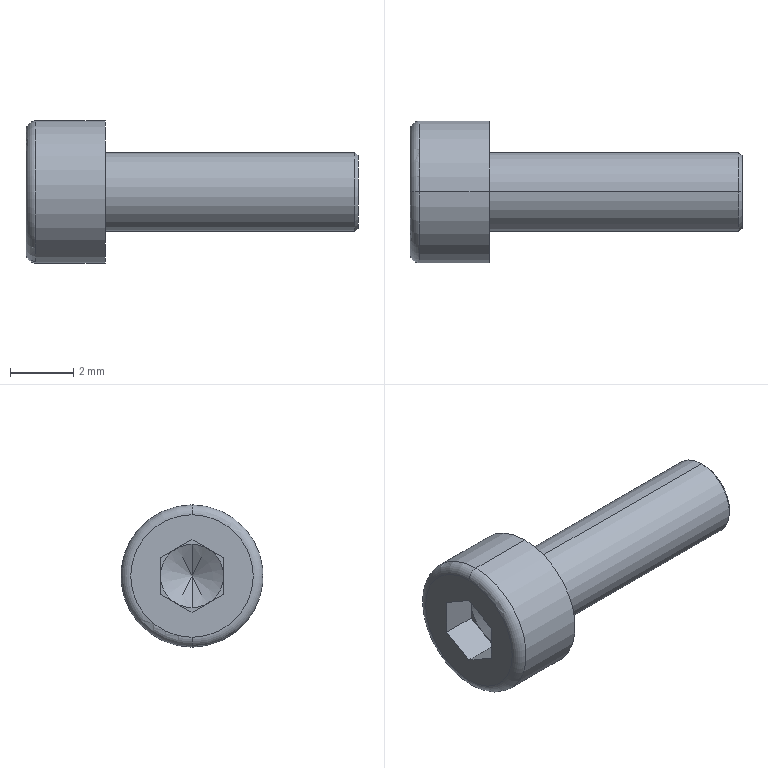Part | STEP file | hexagon socket head cap screws gb_GB_FASTENER_SCREWS_HSHCS M2.5X8-N | 1 solid | 25 faces | box 10.5 x 4.5 x 4.5 mm | volume 74.29 mm3 | plane 15 | cone 4 | cylinder 4 | torus 2 | commonest cylinder face diameters 2.5 x2 4.5 x2
STEP:
#1=CARTESIAN_POINT('',(10.5,0.,-1.15));
#2=VERTEX_POINT('',#1);
#3=CARTESIAN_POINT('',(10.5,0.,1.15));
#4=VERTEX_POINT('',#3);
#5=CARTESIAN_POINT('',(10.5,0.,0.));
#6=DIRECTION('',(1.,0.,0.));
#7=DIRECTION('',(0.,0.,-1.));
#8=AXIS2_PLACEMENT_3D('',#5,#6,#7);
#9=CIRCLE('',#8,1.15);
#10=EDGE_CURVE('',#2,#4,#9,.T.);
#11=ORIENTED_EDGE('',*,*,#10,.F.);
#12=CARTESIAN_POINT('',(10.4,0.,-1.25));
#13=VERTEX_POINT('',#12);
#14=CARTESIAN_POINT('',(10.5,0.,-1.15));
#15=DIRECTION('',(-0.7071,0.,-0.7071));
#16=VECTOR('',#15,1000.);
#17=LINE('',#14,#16);
#18=EDGE_CURVE('',#2,#13,#17,.T.);
#19=ORIENTED_EDGE('',*,*,#18,.T.);
#20=CARTESIAN_POINT('',(10.4,0.,1.25));
#21=VERTEX_POINT('',#20);
#22=CARTESIAN_POINT('',(10.4,0.,0.));
#23=DIRECTION('',(-1.,0.,0.));
#24=DIRECTION('',(0.,0.,-1.));
#25=AXIS2_PLACEMENT_3D('',#22,#23,#24);
#26=CIRCLE('',#25,1.25);
#27=EDGE_CURVE('',#21,#13,#26,.T.);
#28=ORIENTED_EDGE('',*,*,#27,.F.);
#29=CARTESIAN_POINT('',(10.5,0.,1.15));
#30=DIRECTION('',(-0.7071,0.,0.7071));
#31=VECTOR('',#30,1000.);
#32=LINE('',#29,#31);
#33=EDGE_CURVE('',#4,#21,#32,.T.);
#34=ORIENTED_EDGE('',*,*,#33,.F.);
#35=EDGE_LOOP('',(#11,#19,#28,#34));
#36=FACE_OUTER_BOUND('',#35,.T.);
#37=CARTESIAN_POINT('',(10.5,0.,0.));
#38=DIRECTION('',(-1.,0.,0.));
#39=DIRECTION('',(0.,0.,1.));
#40=AXIS2_PLACEMENT_3D('',#37,#38,#39);
#41=CONICAL_SURFACE('',#40,1.15,0.7854);
#42=ADVANCED_FACE('',(#36),#41,.T.);
#43=CARTESIAN_POINT('',(0.,0.,1.938));
#44=VERTEX_POINT('',#43);
#45=CARTESIAN_POINT('',(0.,0.,-1.938));
#46=VERTEX_POINT('',#45);
#47=CARTESIAN_POINT('',(0.,0.,0.));
#48=DIRECTION('',(-1.,0.,0.));
#49=DIRECTION('',(0.,0.,-1.));
#50=AXIS2_PLACEMENT_3D('',#47,#48,#49);
#51=CIRCLE('',#50,1.938);
#52=EDGE_CURVE('',#44,#46,#51,.T.);
#53=ORIENTED_EDGE('',*,*,#52,.F.);
#54=CARTESIAN_POINT('',(0.3125,0.,2.25));
#55=VERTEX_POINT('',#54);
#56=CARTESIAN_POINT('',(0.3125,0.,1.938));
#57=DIRECTION('',(0.,1.,0.));
#58=DIRECTION('',(0.,0.,1.));
#59=AXIS2_PLACEMENT_3D('',#56,#57,#58);
#60=CIRCLE('',#59,0.3125);
#61=EDGE_CURVE('',#44,#55,#60,.T.);
#62=ORIENTED_EDGE('',*,*,#61,.T.);
#63=CARTESIAN_POINT('',(0.3125,0.,-2.25));
#64=VERTEX_POINT('',#63);
#65=CARTESIAN_POINT('',(0.3125,0.,0.));
#66=DIRECTION('',(1.,0.,0.));
#67=DIRECTION('',(0.,0.,-1.));
#68=AXIS2_PLACEMENT_3D('',#65,#66,#67);
#69=CIRCLE('',#68,2.25);
#70=EDGE_CURVE('',#64,#55,#69,.T.);
#71=ORIENTED_EDGE('',*,*,#70,.F.);
#72=CARTESIAN_POINT('',(0.3125,0.,-1.938));
#73=DIRECTION('',(0.,-1.,0.));
#74=DIRECTION('',(0.,0.,-1.));
#75=AXIS2_PLACEMENT_3D('',#72,#73,#74);
#76=CIRCLE('',#75,0.3125);
#77=EDGE_CURVE('',#46,#64,#76,.T.);
#78=ORIENTED_EDGE('',*,*,#77,.F.);
#79=EDGE_LOOP('',(#53,#62,#71,#78));
#80=FACE_OUTER_BOUND('',#79,.T.);
#81=CARTESIAN_POINT('',(0.3125,0.,0.));
#82=DIRECTION('',(1.,0.,0.));
#83=DIRECTION('',(0.,0.,-1.));
#84=AXIS2_PLACEMENT_3D('',#81,#82,#83);
#85=TOROIDAL_SURFACE('',#84,1.938,0.3125);
#86=ADVANCED_FACE('',(#80),#85,.T.);
#87=CARTESIAN_POINT('',(1.677,0.,0.));
#88=VERTEX_POINT('',#87);
#89=CARTESIAN_POINT('',(1.1,0.,1.));
#90=VERTEX_POINT('',#89);
#91=CARTESIAN_POINT('',(1.1,0.,1.));
#92=DIRECTION('',(-0.5,0.,0.866));
#93=VECTOR('',#92,1000.);
#94=LINE('',#91,#93);
#95=EDGE_CURVE('',#88,#90,#94,.T.);
#96=ORIENTED_EDGE('',*,*,#95,.F.);
#97=CARTESIAN_POINT('',(1.1,0.,-1.));
#98=VERTEX_POINT('',#97);
#99=CARTESIAN_POINT('',(1.1,0.,-1.));
#100=DIRECTION('',(-0.5,0.,-0.866));
#101=VECTOR('',#100,1000.);
#102=LINE('',#99,#101);
#103=EDGE_CURVE('',#88,#98,#102,.T.);
#104=ORIENTED_EDGE('',*,*,#103,.T.);
#105=CARTESIAN_POINT('',(1.1,-0.5,-0.866));
#106=VERTEX_POINT('',#105);
#107=CARTESIAN_POINT('',(1.1,0.,0.));
#108=DIRECTION('',(-1.,0.,0.));
#109=DIRECTION('',(0.,0.,-1.));
#110=AXIS2_PLACEMENT_3D('',#107,#108,#109);
#111=CIRCLE('',#110,1.);
#112=EDGE_CURVE('',#98,#106,#111,.T.);
#113=ORIENTED_EDGE('',*,*,#112,.T.);
#114=CARTESIAN_POINT('',(1.1,-1.,0.));
#115=VERTEX_POINT('',#114);
#116=CARTESIAN_POINT('',(1.1,0.,0.));
#117=DIRECTION('',(-1.,0.,0.));
#118=DIRECTION('',(0.,0.,-1.));
#119=AXIS2_PLACEMENT_3D('',#116,#117,#118);
#120=CIRCLE('',#119,1.);
#121=EDGE_CURVE('',#106,#115,#120,.T.);
#122=ORIENTED_EDGE('',*,*,#121,.T.);
#123=CARTESIAN_POINT('',(1.1,-0.5,0.866));
#124=VERTEX_POINT('',#123);
#125=CARTESIAN_POINT('',(1.1,0.,0.));
#126=DIRECTION('',(-1.,0.,0.));
#127=DIRECTION('',(0.,0.,-1.));
#128=AXIS2_PLACEMENT_3D('',#125,#126,#127);
#129=CIRCLE('',#128,1.);
#130=EDGE_CURVE('',#115,#124,#129,.T.);
#131=ORIENTED_EDGE('',*,*,#130,.T.);
#132=CARTESIAN_POINT('',(1.1,0.,0.));
#133=DIRECTION('',(-1.,0.,0.));
#134=DIRECTION('',(0.,0.,-1.));
#135=AXIS2_PLACEMENT_3D('',#132,#133,#134);
#136=CIRCLE('',#135,1.);
#137=EDGE_CURVE('',#124,#90,#136,.T.);
#138=ORIENTED_EDGE('',*,*,#137,.T.);
#139=EDGE_LOOP('',(#96,#104,#113,#122,#131,#138));
#140=FACE_OUTER_BOUND('',#139,.T.);
#141=CARTESIAN_POINT('',(1.1,0.,0.));
#142=DIRECTION('',(-1.,0.,0.));
#143=DIRECTION('',(0.,0.,1.));
#144=AXIS2_PLACEMENT_3D('',#141,#142,#143);
#145=CONICAL_SURFACE('',#144,1.,1.047);
#146=ADVANCED_FACE('',(#140),#145,.F.);
#147=ORIENTED_EDGE('',*,*,#27,.T.);
#148=CARTESIAN_POINT('',(2.5,0.,-1.25));
#149=VERTEX_POINT('',#148);
#150=CARTESIAN_POINT('',(10.5,0.,-1.25));
#151=DIRECTION('',(-1.,0.,0.));
#152=VECTOR('',#151,1000.);
#153=LINE('',#150,#152);
#154=EDGE_CURVE('',#13,#149,#153,.T.);
#155=ORIENTED_EDGE('',*,*,#154,.T.);
#156=CARTESIAN_POINT('',(2.5,0.,1.25));
#157=VERTEX_POINT('',#156);
#158=CARTESIAN_POINT('',(2.5,0.,0.));
#159=DIRECTION('',(1.,0.,0.));
#160=DIRECTION('',(0.,0.,-1.));
#161=AXIS2_PLACEMENT_3D('',#158,#159,#160);
#162=CIRCLE('',#161,1.25);
#163=EDGE_CURVE('',#149,#157,#162,.T.);
#164=ORIENTED_EDGE('',*,*,#163,.T.);
#165=CARTESIAN_POINT('',(10.5,0.,1.25));
#166=DIRECTION('',(-1.,0.,0.));
#167=VECTOR('',#166,1000.);
#168=LINE('',#165,#167);
#169=EDGE_CURVE('',#21,#157,#168,.T.);
#170=ORIENTED_EDGE('',*,*,#169,.F.);
#171=EDGE_LOOP('',(#147,#155,#164,#170));
#172=FACE_OUTER_BOUND('',#171,.T.);
#173=CARTESIAN_POINT('',(10.5,0.,0.));
#174=DIRECTION('',(-1.,0.,0.));
#175=DIRECTION('',(0.,0.,1.));
#176=AXIS2_PLACEMENT_3D('',#173,#174,#175);
#177=CYLINDRICAL_SURFACE('',#176,1.25);
#178=ADVANCED_FACE('',(#172),#177,.T.);
#179=CARTESIAN_POINT('',(2.5,0.,-2.25));
#180=VERTEX_POINT('',#179);
#181=CARTESIAN_POINT('',(2.5,0.,2.25));
#182=VERTEX_POINT('',#181);
#183=CARTESIAN_POINT('',(2.5,0.,0.));
#184=DIRECTION('',(1.,0.,0.));
#185=DIRECTION('',(0.,0.,-1.));
#186=AXIS2_PLACEMENT_3D('',#183,#184,#185);
#187=CIRCLE('',#186,2.25);
#188=EDGE_CURVE('',#180,#182,#187,.T.);
#189=ORIENTED_EDGE('',*,*,#188,.F.);
#190=CARTESIAN_POINT('',(2.5,0.,-2.25));
#191=DIRECTION('',(-1.,0.,0.));
#192=VECTOR('',#191,1000.);
#193=LINE('',#190,#192);
#194=EDGE_CURVE('',#180,#64,#193,.T.);
#195=ORIENTED_EDGE('',*,*,#194,.T.);
#196=ORIENTED_EDGE('',*,*,#70,.T.);
#197=CARTESIAN_POINT('',(2.5,0.,2.25));
#198=DIRECTION('',(-1.,0.,0.));
#199=VECTOR('',#198,1000.);
#200=LINE('',#197,#199);
#201=EDGE_CURVE('',#182,#55,#200,.T.);
#202=ORIENTED_EDGE('',*,*,#201,.F.);
#203=EDGE_LOOP('',(#189,#195,#196,#202));
#204=FACE_OUTER_BOUND('',#203,.T.);
#205=CARTESIAN_POINT('',(2.5,0.,0.));
#206=DIRECTION('',(-1.,0.,0.));
#207=DIRECTION('',(0.,0.,1.));
#208=AXIS2_PLACEMENT_3D('',#205,#206,#207);
#209=CYLINDRICAL_SURFACE('',#208,2.25);
#210=ADVANCED_FACE('',(#204),#209,.T.);
#211=ORIENTED_EDGE('',*,*,#121,.F.);
#212=CARTESIAN_POINT('',(1.1,-1.,-0.5774));
#213=VERTEX_POINT('',#212);
#214=CARTESIAN_POINT('',(1.1,-1.,-0.5774));
#215=DIRECTION('',(0.,0.866,-0.5));
#216=VECTOR('',#215,1000.);
#217=LINE('',#214,#216);
#218=EDGE_CURVE('',#213,#106,#217,.T.);
#219=ORIENTED_EDGE('',*,*,#218,.F.);
#220=CARTESIAN_POINT('',(1.1,-1.,0.5774));
#221=DIRECTION('',(0.,0.,-1.));
#222=VECTOR('',#221,1000.);
#223=LINE('',#220,#222);
#224=EDGE_CURVE('',#115,#213,#223,.T.);
#225=ORIENTED_EDGE('',*,*,#224,.F.);
#226=EDGE_LOOP('',(#211,#219,#225));
#227=FACE_OUTER_BOUND('',#226,.T.);
#228=CARTESIAN_POINT('',(1.1,1.,-1.732));
#229=DIRECTION('',(1.,0.,0.));
#230=DIRECTION('',(0.,0.,-1.));
#231=AXIS2_PLACEMENT_3D('',#228,#229,#230);
#232=PLANE('',#231);
#233=ADVANCED_FACE('',(#227),#232,.F.);
#234=ORIENTED_EDGE('',*,*,#130,.F.);
#235=CARTESIAN_POINT('',(1.1,-1.,0.5774));
#236=VERTEX_POINT('',#235);
#237=CARTESIAN_POINT('',(1.1,-1.,0.5774));
#238=DIRECTION('',(0.,0.,-1.));
#239=VECTOR('',#238,1000.);
#240=LINE('',#237,#239);
#241=EDGE_CURVE('',#236,#115,#240,.T.);
#242=ORIENTED_EDGE('',*,*,#241,.F.);
#243=CARTESIAN_POINT('',(1.1,0.,1.155));
#244=DIRECTION('',(0.,-0.866,-0.5));
#245=VECTOR('',#244,1000.);
#246=LINE('',#243,#245);
#247=EDGE_CURVE('',#124,#236,#246,.T.);
#248=ORIENTED_EDGE('',*,*,#247,.F.);
#249=EDGE_LOOP('',(#234,#242,#248));
#250=FACE_OUTER_BOUND('',#249,.T.);
#251=CARTESIAN_POINT('',(1.1,1.,-1.732));
#252=DIRECTION('',(1.,0.,0.));
#253=DIRECTION('',(0.,0.,-1.));
#254=AXIS2_PLACEMENT_3D('',#251,#252,#253);
#255=PLANE('',#254);
#256=ADVANCED_FACE('',(#250),#255,.F.);
#257=ORIENTED_EDGE('',*,*,#137,.F.);
#258=CARTESIAN_POINT('',(1.1,0.,1.155));
#259=VERTEX_POINT('',#258);
#260=CARTESIAN_POINT('',(1.1,0.,1.155));
#261=DIRECTION('',(0.,-0.866,-0.5));
#262=VECTOR('',#261,1000.);
#263=LINE('',#260,#262);
#264=EDGE_CURVE('',#259,#124,#263,.T.);
#265=ORIENTED_EDGE('',*,*,#264,.F.);
#266=CARTESIAN_POINT('',(1.1,0.5,0.866));
#267=VERTEX_POINT('',#266);
#268=CARTESIAN_POINT('',(1.1,1.,0.5774));
#269=DIRECTION('',(0.,-0.866,0.5));
#270=VECTOR('',#269,1000.);
#271=LINE('',#268,#270);
#272=EDGE_CURVE('',#267,#259,#271,.T.);
#273=ORIENTED_EDGE('',*,*,#272,.F.);
#274=CARTESIAN_POINT('',(1.1,0.,0.));
#275=DIRECTION('',(-1.,0.,0.));
#276=DIRECTION('',(0.,0.,-1.));
#277=AXIS2_PLACEMENT_3D('',#274,#275,#276);
#278=CIRCLE('',#277,1.);
#279=EDGE_CURVE('',#90,#267,#278,.T.);
#280=ORIENTED_EDGE('',*,*,#279,.F.);
#281=EDGE_LOOP('',(#257,#265,#273,#280));
#282=FACE_OUTER_BOUND('',#281,.T.);
#283=CARTESIAN_POINT('',(1.1,1.,-1.732));
#284=DIRECTION('',(1.,0.,0.));
#285=DIRECTION('',(0.,0.,-1.));
#286=AXIS2_PLACEMENT_3D('',#283,#284,#285);
#287=PLANE('',#286);
#288=ADVANCED_FACE('',(#282),#287,.F.);
#289=CARTESIAN_POINT('',(1.1,1.,0.));
#290=VERTEX_POINT('',#289);
#291=CARTESIAN_POINT('',(1.1,0.,0.));
#292=DIRECTION('',(-1.,0.,0.));
#293=DIRECTION('',(0.,0.,-1.));
#294=AXIS2_PLACEMENT_3D('',#291,#292,#293);
#295=CIRCLE('',#294,1.);
#296=EDGE_CURVE('',#267,#290,#295,.T.);
#297=ORIENTED_EDGE('',*,*,#296,.F.);
#298=CARTESIAN_POINT('',(1.1,1.,0.5774));
#299=VERTEX_POINT('',#298);
#300=CARTESIAN_POINT('',(1.1,1.,0.5774));
#301=DIRECTION('',(0.,-0.866,0.5));
#302=VECTOR('',#301,1000.);
#303=LINE('',#300,#302);
#304=EDGE_CURVE('',#299,#267,#303,.T.);
#305=ORIENTED_EDGE('',*,*,#304,.F.);
#306=CARTESIAN_POINT('',(1.1,1.,-0.5774));
#307=DIRECTION('',(0.,0.,1.));
#308=VECTOR('',#307,1000.);
#309=LINE('',#306,#308);
#310=EDGE_CURVE('',#290,#299,#309,.T.);
#311=ORIENTED_EDGE('',*,*,#310,.F.);
#312=EDGE_LOOP('',(#297,#305,#311));
#313=FACE_OUTER_BOUND('',#312,.T.);
#314=CARTESIAN_POINT('',(1.1,1.,-1.732));
#315=DIRECTION('',(1.,0.,0.));
#316=DIRECTION('',(0.,0.,-1.));
#317=AXIS2_PLACEMENT_3D('',#314,#315,#316);
#318=PLANE('',#317);
#319=ADVANCED_FACE('',(#313),#318,.F.);
#320=CARTESIAN_POINT('',(1.1,0.5,-0.866));
#321=VERTEX_POINT('',#320);
#322=CARTESIAN_POINT('',(1.1,0.,0.));
#323=DIRECTION('',(1.,0.,0.));
#324=DIRECTION('',(0.,0.,-1.));
#325=AXIS2_PLACEMENT_3D('',#322,#323,#324);
#326=CIRCLE('',#325,1.);
#327=EDGE_CURVE('',#321,#290,#326,.T.);
#328=ORIENTED_EDGE('',*,*,#327,.T.);
#329=CARTESIAN_POINT('',(1.1,1.,-0.5774));
#330=VERTEX_POINT('',#329);
#331=CARTESIAN_POINT('',(1.1,1.,-0.5774));
#332=DIRECTION('',(0.,0.,1.));
#333=VECTOR('',#332,1000.);
#334=LINE('',#331,#333);
#335=EDGE_CURVE('',#330,#290,#334,.T.);
#336=ORIENTED_EDGE('',*,*,#335,.F.);
#337=CARTESIAN_POINT('',(1.1,0.,-1.155));
#338=DIRECTION('',(0.,0.866,0.5));
#339=VECTOR('',#338,1000.);
#340=LINE('',#337,#339);
#341=EDGE_CURVE('',#321,#330,#340,.T.);
#342=ORIENTED_EDGE('',*,*,#341,.F.);
#343=EDGE_LOOP('',(#328,#336,#342));
#344=FACE_OUTER_BOUND('',#343,.T.);
#345=CARTESIAN_POINT('',(1.1,1.,-1.732));
#346=DIRECTION('',(1.,0.,0.));
#347=DIRECTION('',(0.,0.,-1.));
#348=AXIS2_PLACEMENT_3D('',#345,#346,#347);
#349=PLANE('',#348);
#350=ADVANCED_FACE('',(#344),#349,.F.);
#351=CARTESIAN_POINT('',(1.1,0.,0.));
#352=DIRECTION('',(-1.,0.,0.));
#353=DIRECTION('',(0.,0.,-1.));
#354=AXIS2_PLACEMENT_3D('',#351,#352,#353);
#355=CIRCLE('',#354,1.);
#356=EDGE_CURVE('',#321,#98,#355,.T.);
#357=ORIENTED_EDGE('',*,*,#356,.F.);
#358=CARTESIAN_POINT('',(1.1,0.,-1.155));
#359=VERTEX_POINT('',#358);
#360=CARTESIAN_POINT('',(1.1,0.,-1.155));
#361=DIRECTION('',(0.,0.866,0.5));
#362=VECTOR('',#361,1000.);
#363=LINE('',#360,#362);
#364=EDGE_CURVE('',#359,#321,#363,.T.);
#365=ORIENTED_EDGE('',*,*,#364,.F.);
#366=CARTESIAN_POINT('',(1.1,-1.,-0.5774));
#367=DIRECTION('',(0.,0.866,-0.5));
#368=VECTOR('',#367,1000.);
#369=LINE('',#366,#368);
#370=EDGE_CURVE('',#106,#359,#369,.T.);
#371=ORIENTED_EDGE('',*,*,#370,.F.);
#372=ORIENTED_EDGE('',*,*,#112,.F.);
#373=EDGE_LOOP('',(#357,#365,#371,#372));
#374=FACE_OUTER_BOUND('',#373,.T.);
#375=CARTESIAN_POINT('',(1.1,1.,-1.732));
#376=DIRECTION('',(1.,0.,0.));
#377=DIRECTION('',(0.,0.,-1.));
#378=AXIS2_PLACEMENT_3D('',#375,#376,#377);
#379=PLANE('',#378);
#380=ADVANCED_FACE('',(#374),#379,.F.);
#381=CARTESIAN_POINT('',(0.,0.,0.));
#382=DIRECTION('',(-1.,0.,0.));
#383=DIRECTION('',(0.,0.,-1.));
#384=AXIS2_PLACEMENT_3D('',#381,#382,#383);
#385=CIRCLE('',#384,1.938);
#386=EDGE_CURVE('',#46,#44,#385,.T.);
#387=ORIENTED_EDGE('',*,*,#386,.T.);
#388=ORIENTED_EDGE('',*,*,#52,.T.);
#389=EDGE_LOOP('',(#387,#388));
#390=FACE_OUTER_BOUND('',#389,.T.);
#391=CARTESIAN_POINT('',(0.,-1.,-0.5774));
#392=VERTEX_POINT('',#391);
#393=CARTESIAN_POINT('',(0.,0.,-1.155));
#394=VERTEX_POINT('',#393);
#395=CARTESIAN_POINT('',(0.,-1.,-0.5774));
#396=DIRECTION('',(0.,0.866,-0.5));
#397=VECTOR('',#396,1000.);
#398=LINE('',#395,#397);
#399=EDGE_CURVE('',#392,#394,#398,.T.);
#400=ORIENTED_EDGE('',*,*,#399,.T.);
#401=CARTESIAN_POINT('',(0.,1.,-0.5774));
#402=VERTEX_POINT('',#401);
#403=CARTESIAN_POINT('',(0.,0.,-1.155));
#404=DIRECTION('',(0.,0.866,0.5));
#405=VECTOR('',#404,1000.);
#406=LINE('',#403,#405);
#407=EDGE_CURVE('',#394,#402,#406,.T.);
#408=ORIENTED_EDGE('',*,*,#407,.T.);
#409=CARTESIAN_POINT('',(0.,1.,0.5774));
#410=VERTEX_POINT('',#409);
#411=CARTESIAN_POINT('',(0.,1.,-0.5774));
#412=DIRECTION('',(0.,0.,1.));
#413=VECTOR('',#412,1000.);
#414=LINE('',#411,#413);
#415=EDGE_CURVE('',#402,#410,#414,.T.);
#416=ORIENTED_EDGE('',*,*,#415,.T.);
#417=CARTESIAN_POINT('',(0.,0.,1.155));
#418=VERTEX_POINT('',#417);
#419=CARTESIAN_POINT('',(0.,1.,0.5774));
#420=DIRECTION('',(0.,-0.866,0.5));
#421=VECTOR('',#420,1000.);
#422=LINE('',#419,#421);
#423=EDGE_CURVE('',#410,#418,#422,.T.);
#424=ORIENTED_EDGE('',*,*,#423,.T.);
#425=CARTESIAN_POINT('',(0.,-1.,0.5774));
#426=VERTEX_POINT('',#425);
#427=CARTESIAN_POINT('',(0.,0.,1.155));
#428=DIRECTION('',(0.,-0.866,-0.5));
#429=VECTOR('',#428,1000.);
#430=LINE('',#427,#429);
#431=EDGE_CURVE('',#418,#426,#430,.T.);
#432=ORIENTED_EDGE('',*,*,#431,.T.);
#433=CARTESIAN_POINT('',(0.,-1.,0.5774));
#434=DIRECTION('',(0.,0.,-1.));
#435=VECTOR('',#434,1000.);
#436=LINE('',#433,#435);
#437=EDGE_CURVE('',#426,#392,#436,.T.);
#438=ORIENTED_EDGE('',*,*,#437,.T.);
#439=EDGE_LOOP('',(#400,#408,#416,#424,#432,#438));
#440=FACE_BOUND('',#439,.T.);
#441=CARTESIAN_POINT('',(0.,0.,0.));
#442=DIRECTION('',(1.,0.,0.));
#443=DIRECTION('',(0.,0.,-1.));
#444=AXIS2_PLACEMENT_3D('',#441,#442,#443);
#445=PLANE('',#444);
#446=ADVANCED_FACE('',(#390,#440),#445,.F.);
#447=CARTESIAN_POINT('',(2.5,0.,0.));
#448=DIRECTION('',(1.,0.,0.));
#449=DIRECTION('',(0.,0.,-1.));
#450=AXIS2_PLACEMENT_3D('',#447,#448,#449);
#451=CIRCLE('',#450,2.25);
#452=EDGE_CURVE('',#182,#180,#451,.T.);
#453=ORIENTED_EDGE('',*,*,#452,.T.);
#454=ORIENTED_EDGE('',*,*,#188,.T.);
#455=EDGE_LOOP('',(#453,#454));
#456=FACE_OUTER_BOUND('',#455,.T.);
#457=CARTESIAN_POINT('',(2.5,0.,0.));
#458=DIRECTION('',(1.,0.,0.));
#459=DIRECTION('',(0.,0.,-1.));
#460=AXIS2_PLACEMENT_3D('',#457,#458,#459);
#461=CIRCLE('',#460,1.25);
#462=EDGE_CURVE('',#157,#149,#461,.T.);
#463=ORIENTED_EDGE('',*,*,#462,.F.);
#464=ORIENTED_EDGE('',*,*,#163,.F.);
#465=EDGE_LOOP('',(#463,#464));
#466=FACE_BOUND('',#465,.T.);
#467=CARTESIAN_POINT('',(2.5,0.,0.));
#468=DIRECTION('',(1.,0.,0.));
#469=DIRECTION('',(0.,0.,-1.));
#470=AXIS2_PLACEMENT_3D('',#467,#468,#469);
#471=PLANE('',#470);
#472=ADVANCED_FACE('',(#456,#466),#471,.T.);
#473=ORIENTED_EDGE('',*,*,#194,.F.);
#474=ORIENTED_EDGE('',*,*,#452,.F.);
#475=ORIENTED_EDGE('',*,*,#201,.T.);
#476=CARTESIAN_POINT('',(0.3125,0.,0.));
#477=DIRECTION('',(1.,0.,0.));
#478=DIRECTION('',(0.,0.,-1.));
#479=AXIS2_PLACEMENT_3D('',#476,#477,#478);
#480=CIRCLE('',#479,2.25);
#481=EDGE_CURVE('',#55,#64,#480,.T.);
#482=ORIENTED_EDGE('',*,*,#481,.T.);
#483=EDGE_LOOP('',(#473,#474,#475,#482));
#484=FACE_OUTER_BOUND('',#483,.T.);
#485=CARTESIAN_POINT('',(2.5,0.,0.));
#486=DIRECTION('',(-1.,0.,0.));
#487=DIRECTION('',(0.,0.,1.));
#488=AXIS2_PLACEMENT_3D('',#485,#486,#487);
#489=CYLINDRICAL_SURFACE('',#488,2.25);
#490=ADVANCED_FACE('',(#484),#489,.T.);
#491=ORIENTED_EDGE('',*,*,#154,.F.);
#492=CARTESIAN_POINT('',(10.4,0.,0.));
#493=DIRECTION('',(-1.,0.,0.));
#494=DIRECTION('',(0.,0.,-1.));
#495=AXIS2_PLACEMENT_3D('',#492,#493,#494);
#496=CIRCLE('',#495,1.25);
#497=EDGE_CURVE('',#13,#21,#496,.T.);
#498=ORIENTED_EDGE('',*,*,#497,.T.);
#499=ORIENTED_EDGE('',*,*,#169,.T.);
#500=ORIENTED_EDGE('',*,*,#462,.T.);
#501=EDGE_LOOP('',(#491,#498,#499,#500));
#502=FACE_OUTER_BOUND('',#501,.T.);
#503=CARTESIAN_POINT('',(10.5,0.,0.));
#504=DIRECTION('',(-1.,0.,0.));
#505=DIRECTION('',(0.,0.,1.));
#506=AXIS2_PLACEMENT_3D('',#503,#504,#505);
#507=CYLINDRICAL_SURFACE('',#506,1.25);
#508=ADVANCED_FACE('',(#502),#507,.T.);
#509=CARTESIAN_POINT('',(10.5,0.,0.));
#510=DIRECTION('',(1.,0.,0.));
#511=DIRECTION('',(0.,0.,-1.));
#512=AXIS2_PLACEMENT_3D('',#509,#510,#511);
#513=CIRCLE('',#512,1.15);
#514=EDGE_CURVE('',#4,#2,#513,.T.);
#515=ORIENTED_EDGE('',*,*,#514,.T.);
#516=ORIENTED_EDGE('',*,*,#10,.T.);
#517=EDGE_LOOP('',(#515,#516));
#518=FACE_OUTER_BOUND('',#517,.T.);
#519=CARTESIAN_POINT('',(10.5,0.,0.));
#520=DIRECTION('',(1.,0.,0.));
#521=DIRECTION('',(0.,0.,-1.));
#522=AXIS2_PLACEMENT_3D('',#519,#520,#521);
#523=PLANE('',#522);
#524=ADVANCED_FACE('',(#518),#523,.T.);
#525=ORIENTED_EDGE('',*,*,#399,.F.);
#526=CARTESIAN_POINT('',(1.1,-1.,-0.5774));
#527=DIRECTION('',(-1.,0.,0.));
#528=VECTOR('',#527,1000.);
#529=LINE('',#526,#528);
#530=EDGE_CURVE('',#213,#392,#529,.T.);
#531=ORIENTED_EDGE('',*,*,#530,.F.);
#532=ORIENTED_EDGE('',*,*,#218,.T.);
#533=ORIENTED_EDGE('',*,*,#370,.T.);
#534=CARTESIAN_POINT('',(1.1,0.,-1.155));
#535=DIRECTION('',(-1.,0.,0.));
#536=VECTOR('',#535,1000.);
#537=LINE('',#534,#536);
#538=EDGE_CURVE('',#359,#394,#537,.T.);
#539=ORIENTED_EDGE('',*,*,#538,.T.);
#540=EDGE_LOOP('',(#525,#531,#532,#533,#539));
#541=FACE_OUTER_BOUND('',#540,.T.);
#542=CARTESIAN_POINT('',(1.1,-1.,-0.5774));
#543=DIRECTION('',(0.,0.5,0.866));
#544=DIRECTION('',(0.,-0.866,0.5));
#545=AXIS2_PLACEMENT_3D('',#542,#543,#544);
#546=PLANE('',#545);
#547=ADVANCED_FACE('',(#541),#546,.T.);
#548=ORIENTED_EDGE('',*,*,#407,.F.);
#549=ORIENTED_EDGE('',*,*,#538,.F.);
#550=ORIENTED_EDGE('',*,*,#364,.T.);
#551=ORIENTED_EDGE('',*,*,#341,.T.);
#552=CARTESIAN_POINT('',(1.1,1.,-0.5774));
#553=DIRECTION('',(-1.,0.,0.));
#554=VECTOR('',#553,1000.);
#555=LINE('',#552,#554);
#556=EDGE_CURVE('',#330,#402,#555,.T.);
#557=ORIENTED_EDGE('',*,*,#556,.T.);
#558=EDGE_LOOP('',(#548,#549,#550,#551,#557));
#559=FACE_OUTER_BOUND('',#558,.T.);
#560=CARTESIAN_POINT('',(1.1,0.,-1.155));
#561=DIRECTION('',(0.,-0.5,0.866));
#562=DIRECTION('',(0.,-0.866,-0.5));
#563=AXIS2_PLACEMENT_3D('',#560,#561,#562);
#564=PLANE('',#563);
#565=ADVANCED_FACE('',(#559),#564,.T.);
#566=ORIENTED_EDGE('',*,*,#415,.F.);
#567=ORIENTED_EDGE('',*,*,#556,.F.);
#568=ORIENTED_EDGE('',*,*,#335,.T.);
#569=ORIENTED_EDGE('',*,*,#310,.T.);
#570=CARTESIAN_POINT('',(1.1,1.,0.5774));
#571=DIRECTION('',(-1.,0.,0.));
#572=VECTOR('',#571,1000.);
#573=LINE('',#570,#572);
#574=EDGE_CURVE('',#299,#410,#573,.T.);
#575=ORIENTED_EDGE('',*,*,#574,.T.);
#576=EDGE_LOOP('',(#566,#567,#568,#569,#575));
#577=FACE_OUTER_BOUND('',#576,.T.);
#578=CARTESIAN_POINT('',(1.1,1.,-0.5774));
#579=DIRECTION('',(0.,-1.,0.));
#580=DIRECTION('',(0.,0.,-1.));
#581=AXIS2_PLACEMENT_3D('',#578,#579,#580);
#582=PLANE('',#581);
#583=ADVANCED_FACE('',(#577),#582,.T.);
#584=ORIENTED_EDGE('',*,*,#423,.F.);
#585=ORIENTED_EDGE('',*,*,#574,.F.);
#586=ORIENTED_EDGE('',*,*,#304,.T.);
#587=ORIENTED_EDGE('',*,*,#272,.T.);
#588=CARTESIAN_POINT('',(1.1,0.,1.155));
#589=DIRECTION('',(-1.,0.,0.));
#590=VECTOR('',#589,1000.);
#591=LINE('',#588,#590);
#592=EDGE_CURVE('',#259,#418,#591,.T.);
#593=ORIENTED_EDGE('',*,*,#592,.T.);
#594=EDGE_LOOP('',(#584,#585,#586,#587,#593));
#595=FACE_OUTER_BOUND('',#594,.T.);
#596=CARTESIAN_POINT('',(1.1,1.,0.5774));
#597=DIRECTION('',(0.,-0.5,-0.866));
#598=DIRECTION('',(0.,0.866,-0.5));
#599=AXIS2_PLACEMENT_3D('',#596,#597,#598);
#600=PLANE('',#599);
#601=ADVANCED_FACE('',(#595),#600,.T.);
#602=ORIENTED_EDGE('',*,*,#431,.F.);
#603=ORIENTED_EDGE('',*,*,#592,.F.);
#604=ORIENTED_EDGE('',*,*,#264,.T.);
#605=ORIENTED_EDGE('',*,*,#247,.T.);
#606=CARTESIAN_POINT('',(1.1,-1.,0.5774));
#607=DIRECTION('',(-1.,0.,0.));
#608=VECTOR('',#607,1000.);
#609=LINE('',#606,#608);
#610=EDGE_CURVE('',#236,#426,#609,.T.);
#611=ORIENTED_EDGE('',*,*,#610,.T.);
#612=EDGE_LOOP('',(#602,#603,#604,#605,#611));
#613=FACE_OUTER_BOUND('',#612,.T.);
#614=CARTESIAN_POINT('',(1.1,0.,1.155));
#615=DIRECTION('',(0.,0.5,-0.866));
#616=DIRECTION('',(0.,0.866,0.5));
#617=AXIS2_PLACEMENT_3D('',#614,#615,#616);
#618=PLANE('',#617);
#619=ADVANCED_FACE('',(#613),#618,.T.);
#620=ORIENTED_EDGE('',*,*,#437,.F.);
#621=ORIENTED_EDGE('',*,*,#610,.F.);
#622=ORIENTED_EDGE('',*,*,#241,.T.);
#623=ORIENTED_EDGE('',*,*,#224,.T.);
#624=ORIENTED_EDGE('',*,*,#530,.T.);
#625=EDGE_LOOP('',(#620,#621,#622,#623,#624));
#626=FACE_OUTER_BOUND('',#625,.T.);
#627=CARTESIAN_POINT('',(1.1,-1.,0.5774));
#628=DIRECTION('',(0.,1.,0.));
#629=DIRECTION('',(0.,0.,1.));
#630=AXIS2_PLACEMENT_3D('',#627,#628,#629);
#631=PLANE('',#630);
#632=ADVANCED_FACE('',(#626),#631,.T.);
#633=ORIENTED_EDGE('',*,*,#103,.F.);
#634=ORIENTED_EDGE('',*,*,#95,.T.);
#635=ORIENTED_EDGE('',*,*,#279,.T.);
#636=ORIENTED_EDGE('',*,*,#296,.T.);
#637=ORIENTED_EDGE('',*,*,#327,.F.);
#638=ORIENTED_EDGE('',*,*,#356,.T.);
#639=EDGE_LOOP('',(#633,#634,#635,#636,#637,#638));
#640=FACE_OUTER_BOUND('',#639,.T.);
#641=CARTESIAN_POINT('',(1.1,0.,0.));
#642=DIRECTION('',(-1.,0.,0.));
#643=DIRECTION('',(0.,0.,1.));
#644=AXIS2_PLACEMENT_3D('',#641,#642,#643);
#645=CONICAL_SURFACE('',#644,1.,1.047);
#646=ADVANCED_FACE('',(#640),#645,.F.);
#647=ORIENTED_EDGE('',*,*,#61,.F.);
#648=ORIENTED_EDGE('',*,*,#386,.F.);
#649=ORIENTED_EDGE('',*,*,#77,.T.);
#650=ORIENTED_EDGE('',*,*,#481,.F.);
#651=EDGE_LOOP('',(#647,#648,#649,#650));
#652=FACE_OUTER_BOUND('',#651,.T.);
#653=CARTESIAN_POINT('',(0.3125,0.,0.));
#654=DIRECTION('',(1.,0.,0.));
#655=DIRECTION('',(0.,0.,-1.));
#656=AXIS2_PLACEMENT_3D('',#653,#654,#655);
#657=TOROIDAL_SURFACE('',#656,1.938,0.3125);
#658=ADVANCED_FACE('',(#652),#657,.T.);
#659=ORIENTED_EDGE('',*,*,#18,.F.);
#660=ORIENTED_EDGE('',*,*,#514,.F.);
#661=ORIENTED_EDGE('',*,*,#33,.T.);
#662=ORIENTED_EDGE('',*,*,#497,.F.);
#663=EDGE_LOOP('',(#659,#660,#661,#662));
#664=FACE_OUTER_BOUND('',#663,.T.);
#665=CARTESIAN_POINT('',(10.5,0.,0.));
#666=DIRECTION('',(-1.,0.,0.));
#667=DIRECTION('',(0.,0.,1.));
#668=AXIS2_PLACEMENT_3D('',#665,#666,#667);
#669=CONICAL_SURFACE('',#668,1.15,0.7854);
#670=ADVANCED_FACE('',(#664),#669,.T.);
#671=CLOSED_SHELL('',(#42,#86,#146,#178,#210,#233,#256,#288,#319,#350,#380,#446,#472,#490,#508,#524,#547,#565,#583,#601,#619,#632,#646,#658,#670));
#672=MANIFOLD_SOLID_BREP('',#671);
#673=CARTESIAN_POINT('',(0.,0.,0.));
#674=DIRECTION('',(0.,0.,1.));
#675=DIRECTION('',(1.,0.,0.));
#676=AXIS2_PLACEMENT_3D('',#673,#674,#675);
#677=(LENGTH_UNIT()NAMED_UNIT(*)SI_UNIT(.MILLI.,.METRE.));
#678=UNCERTAINTY_MEASURE_WITH_UNIT(LENGTH_MEASURE(0.00001),#677,'','');
#679=(NAMED_UNIT(*)PLANE_ANGLE_UNIT()SI_UNIT($,.RADIAN.));
#680=(NAMED_UNIT(*)SI_UNIT($,.STERADIAN.)SOLID_ANGLE_UNIT());
#681=(GEOMETRIC_REPRESENTATION_CONTEXT(3)GLOBAL_UNCERTAINTY_ASSIGNED_CONTEXT((#678))GLOBAL_UNIT_ASSIGNED_CONTEXT((#677,#679,#680))REPRESENTATION_CONTEXT('',''));
#682=ADVANCED_BREP_SHAPE_REPRESENTATION('',(#672,#676),#681);